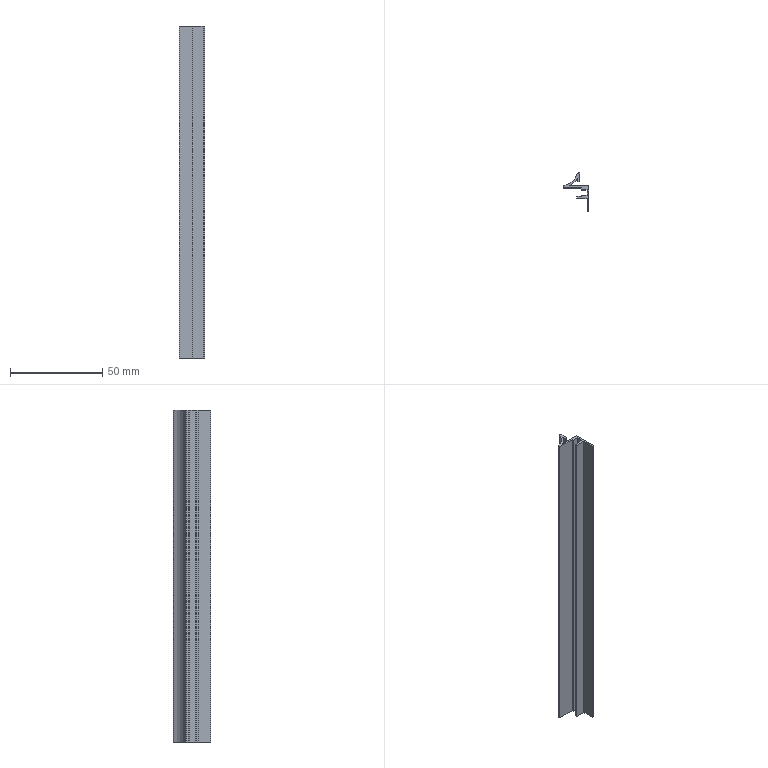Part | SolidWorks | features BaseBody 1, ICE 1, MoveFace 1 | 1 solid | 27 faces | box 14 x 20.3 x 180 mm | volume 9165 mm3 | plane 20 | cylinder 7 | commonest cylinder face diameters 0.387 x2 0.8 x2 0.4 x1 20 x1 22 x1
STEP:
#1=CARTESIAN_POINT('',(-5.304,-0.625,200.));
#2=VERTEX_POINT('',#1);
#3=CARTESIAN_POINT('',(-5.449,-0.8125,200.));
#4=VERTEX_POINT('',#3);
#5=CARTESIAN_POINT('',(-5.255,-0.8125,200.));
#6=DIRECTION('',(0.,0.,1.));
#7=DIRECTION('',(-1.,0.,0.));
#8=AXIS2_PLACEMENT_3D('',#5,#6,#7);
#9=CIRCLE('',#8,0.1937);
#10=EDGE_CURVE('',#2,#4,#9,.T.);
#11=ORIENTED_EDGE('',*,*,#10,.T.);
#12=CARTESIAN_POINT('',(-5.449,-0.8125,20.));
#13=VERTEX_POINT('',#12);
#14=CARTESIAN_POINT('',(-5.449,-0.8125,230.));
#15=DIRECTION('',(0.,0.,-1.));
#16=VECTOR('',#15,1000.);
#17=LINE('',#14,#16);
#18=EDGE_CURVE('',#4,#13,#17,.T.);
#19=ORIENTED_EDGE('',*,*,#18,.T.);
#20=CARTESIAN_POINT('',(-5.304,-0.625,20.));
#21=VERTEX_POINT('',#20);
#22=CARTESIAN_POINT('',(-5.255,-0.8125,20.));
#23=DIRECTION('',(0.,0.,-1.));
#24=DIRECTION('',(1.,0.,0.));
#25=AXIS2_PLACEMENT_3D('',#22,#23,#24);
#26=CIRCLE('',#25,0.1937);
#27=EDGE_CURVE('',#13,#21,#26,.T.);
#28=ORIENTED_EDGE('',*,*,#27,.T.);
#29=CARTESIAN_POINT('',(-5.304,-0.625,230.));
#30=DIRECTION('',(0.,0.,-1.));
#31=VECTOR('',#30,1000.);
#32=LINE('',#29,#31);
#33=EDGE_CURVE('',#2,#21,#32,.T.);
#34=ORIENTED_EDGE('',*,*,#33,.F.);
#35=EDGE_LOOP('',(#11,#19,#28,#34));
#36=FACE_OUTER_BOUND('',#35,.T.);
#37=CARTESIAN_POINT('',(-5.255,-0.8125,230.));
#38=DIRECTION('',(0.,0.,-1.));
#39=DIRECTION('',(-1.,0.,0.));
#40=AXIS2_PLACEMENT_3D('',#37,#38,#39);
#41=CYLINDRICAL_SURFACE('',#40,0.1937);
#42=ADVANCED_FACE('',(#36),#41,.F.);
#43=CARTESIAN_POINT('',(5.,-1.,20.));
#44=VERTEX_POINT('',#43);
#45=CARTESIAN_POINT('',(5.,-14.3,20.));
#46=VERTEX_POINT('',#45);
#47=CARTESIAN_POINT('',(5.,29.623,20.));
#48=DIRECTION('',(0.,-1.,0.));
#49=VECTOR('',#48,1000.);
#50=LINE('',#47,#49);
#51=EDGE_CURVE('',#44,#46,#50,.T.);
#52=ORIENTED_EDGE('',*,*,#51,.F.);
#53=CARTESIAN_POINT('',(5.,-1.,200.));
#54=VERTEX_POINT('',#53);
#55=CARTESIAN_POINT('',(5.,-1.,230.));
#56=DIRECTION('',(0.,0.,-1.));
#57=VECTOR('',#56,1000.);
#58=LINE('',#55,#57);
#59=EDGE_CURVE('',#54,#44,#58,.T.);
#60=ORIENTED_EDGE('',*,*,#59,.F.);
#61=CARTESIAN_POINT('',(5.,-14.3,200.));
#62=VERTEX_POINT('',#61);
#63=CARTESIAN_POINT('',(5.,-14.3,200.));
#64=DIRECTION('',(0.,1.,0.));
#65=VECTOR('',#64,1000.);
#66=LINE('',#63,#65);
#67=EDGE_CURVE('',#62,#54,#66,.T.);
#68=ORIENTED_EDGE('',*,*,#67,.F.);
#69=CARTESIAN_POINT('',(5.,-14.3,230.));
#70=DIRECTION('',(0.,0.,1.));
#71=VECTOR('',#70,1000.);
#72=LINE('',#69,#71);
#73=EDGE_CURVE('',#46,#62,#72,.T.);
#74=ORIENTED_EDGE('',*,*,#73,.F.);
#75=EDGE_LOOP('',(#52,#60,#68,#74));
#76=FACE_OUTER_BOUND('',#75,.T.);
#77=CARTESIAN_POINT('',(5.,-14.3,230.));
#78=DIRECTION('',(-1.,0.,0.));
#79=DIRECTION('',(0.,0.,1.));
#80=AXIS2_PLACEMENT_3D('',#77,#78,#79);
#81=PLANE('',#80);
#82=ADVANCED_FACE('',(#76),#81,.F.);
#83=CARTESIAN_POINT('',(-9.,-2.,20.));
#84=VERTEX_POINT('',#83);
#85=CARTESIAN_POINT('',(-9.,-2.,200.));
#86=VERTEX_POINT('',#85);
#87=CARTESIAN_POINT('',(-9.,-2.,230.));
#88=DIRECTION('',(0.,0.,1.));
#89=VECTOR('',#88,1000.);
#90=LINE('',#87,#89);
#91=EDGE_CURVE('',#84,#86,#90,.T.);
#92=ORIENTED_EDGE('',*,*,#91,.F.);
#93=CARTESIAN_POINT('',(0.9,-2.,20.));
#94=VERTEX_POINT('',#93);
#95=CARTESIAN_POINT('',(5.,-2.,20.));
#96=DIRECTION('',(-1.,0.,0.));
#97=VECTOR('',#96,1000.);
#98=LINE('',#95,#97);
#99=EDGE_CURVE('',#94,#84,#98,.T.);
#100=ORIENTED_EDGE('',*,*,#99,.F.);
#101=CARTESIAN_POINT('',(0.9,-2.,200.));
#102=VERTEX_POINT('',#101);
#103=CARTESIAN_POINT('',(0.9,-2.,230.));
#104=DIRECTION('',(0.,0.,-1.));
#105=VECTOR('',#104,1000.);
#106=LINE('',#103,#105);
#107=EDGE_CURVE('',#102,#94,#106,.T.);
#108=ORIENTED_EDGE('',*,*,#107,.F.);
#109=CARTESIAN_POINT('',(5.,-2.,200.));
#110=DIRECTION('',(1.,0.,0.));
#111=VECTOR('',#110,1000.);
#112=LINE('',#109,#111);
#113=EDGE_CURVE('',#86,#102,#112,.T.);
#114=ORIENTED_EDGE('',*,*,#113,.F.);
#115=EDGE_LOOP('',(#92,#100,#108,#114));
#116=FACE_OUTER_BOUND('',#115,.T.);
#117=CARTESIAN_POINT('',(-9.,-2.,230.));
#118=DIRECTION('',(0.,1.,0.));
#119=DIRECTION('',(0.,0.,1.));
#120=AXIS2_PLACEMENT_3D('',#117,#118,#119);
#121=PLANE('',#120);
#122=ADVANCED_FACE('',(#116),#121,.F.);
#123=CARTESIAN_POINT('',(4.,-6.,200.));
#124=VERTEX_POINT('',#123);
#125=CARTESIAN_POINT('',(4.,-3.,200.));
#126=VERTEX_POINT('',#125);
#127=CARTESIAN_POINT('',(4.,29.623,200.));
#128=DIRECTION('',(0.,1.,0.));
#129=VECTOR('',#128,1000.);
#130=LINE('',#127,#129);
#131=EDGE_CURVE('',#124,#126,#130,.T.);
#132=ORIENTED_EDGE('',*,*,#131,.F.);
#133=CARTESIAN_POINT('',(1.,-6.,200.));
#134=VERTEX_POINT('',#133);
#135=CARTESIAN_POINT('',(5.,-6.,200.));
#136=DIRECTION('',(1.,0.,0.));
#137=VECTOR('',#136,1000.);
#138=LINE('',#135,#137);
#139=EDGE_CURVE('',#134,#124,#138,.T.);
#140=ORIENTED_EDGE('',*,*,#139,.F.);
#141=CARTESIAN_POINT('',(1.,-6.7,200.));
#142=VERTEX_POINT('',#141);
#143=CARTESIAN_POINT('',(1.,-6.,200.));
#144=DIRECTION('',(0.,-1.,0.));
#145=VECTOR('',#144,1000.);
#146=LINE('',#143,#145);
#147=EDGE_CURVE('',#134,#142,#146,.T.);
#148=ORIENTED_EDGE('',*,*,#147,.T.);
#149=CARTESIAN_POINT('',(-1.7,-6.7,200.));
#150=VERTEX_POINT('',#149);
#151=CARTESIAN_POINT('',(5.,-6.7,200.));
#152=DIRECTION('',(1.,0.,0.));
#153=VECTOR('',#152,1000.);
#154=LINE('',#151,#153);
#155=EDGE_CURVE('',#150,#142,#154,.T.);
#156=ORIENTED_EDGE('',*,*,#155,.F.);
#157=CARTESIAN_POINT('',(-1.7,-7.7,200.));
#158=VERTEX_POINT('',#157);
#159=CARTESIAN_POINT('',(-1.7,-6.7,200.));
#160=DIRECTION('',(0.,-1.,0.));
#161=VECTOR('',#160,1000.);
#162=LINE('',#159,#161);
#163=EDGE_CURVE('',#150,#158,#162,.T.);
#164=ORIENTED_EDGE('',*,*,#163,.T.);
#165=CARTESIAN_POINT('',(4.,-7.7,200.));
#166=VERTEX_POINT('',#165);
#167=CARTESIAN_POINT('',(5.,-7.7,200.));
#168=DIRECTION('',(-1.,0.,0.));
#169=VECTOR('',#168,1000.);
#170=LINE('',#167,#169);
#171=EDGE_CURVE('',#166,#158,#170,.T.);
#172=ORIENTED_EDGE('',*,*,#171,.F.);
#173=CARTESIAN_POINT('',(4.,-14.3,200.));
#174=VERTEX_POINT('',#173);
#175=CARTESIAN_POINT('',(4.,29.623,200.));
#176=DIRECTION('',(0.,1.,0.));
#177=VECTOR('',#176,1000.);
#178=LINE('',#175,#177);
#179=EDGE_CURVE('',#174,#166,#178,.T.);
#180=ORIENTED_EDGE('',*,*,#179,.F.);
#181=CARTESIAN_POINT('',(5.,-14.3,200.));
#182=DIRECTION('',(-1.,0.,0.));
#183=VECTOR('',#182,1000.);
#184=LINE('',#181,#183);
#185=EDGE_CURVE('',#62,#174,#184,.T.);
#186=ORIENTED_EDGE('',*,*,#185,.F.);
#187=ORIENTED_EDGE('',*,*,#67,.T.);
#188=CARTESIAN_POINT('',(-5.207,-1.,200.));
#189=VERTEX_POINT('',#188);
#190=CARTESIAN_POINT('',(5.,-1.,200.));
#191=DIRECTION('',(1.,0.,0.));
#192=VECTOR('',#191,1000.);
#193=LINE('',#190,#192);
#194=EDGE_CURVE('',#189,#54,#193,.T.);
#195=ORIENTED_EDGE('',*,*,#194,.F.);
#196=CARTESIAN_POINT('',(-5.255,-0.8125,200.));
#197=DIRECTION('',(0.,0.,1.));
#198=DIRECTION('',(-1.,0.,0.));
#199=AXIS2_PLACEMENT_3D('',#196,#197,#198);
#200=CIRCLE('',#199,0.1937);
#201=EDGE_CURVE('',#4,#189,#200,.T.);
#202=ORIENTED_EDGE('',*,*,#201,.F.);
#203=ORIENTED_EDGE('',*,*,#10,.F.);
#204=CARTESIAN_POINT('',(-1.368,3.063,200.));
#205=VERTEX_POINT('',#204);
#206=CARTESIAN_POINT('',(-10.628,9.,200.));
#207=DIRECTION('',(0.,0.,1.));
#208=DIRECTION('',(-1.,0.,0.));
#209=AXIS2_PLACEMENT_3D('',#206,#207,#208);
#210=CIRCLE('',#209,11.);
#211=EDGE_CURVE('',#2,#205,#210,.T.);
#212=ORIENTED_EDGE('',*,*,#211,.T.);
#213=CARTESIAN_POINT('',(-1.,2.955,200.));
#214=VERTEX_POINT('',#213);
#215=CARTESIAN_POINT('',(-1.2,2.955,200.));
#216=DIRECTION('',(0.,0.,1.));
#217=DIRECTION('',(-1.,0.,0.));
#218=AXIS2_PLACEMENT_3D('',#215,#216,#217);
#219=CIRCLE('',#218,0.2);
#220=EDGE_CURVE('',#214,#205,#219,.T.);
#221=ORIENTED_EDGE('',*,*,#220,.F.);
#222=CARTESIAN_POINT('',(-1.,1.5,200.));
#223=VERTEX_POINT('',#222);
#224=CARTESIAN_POINT('',(-1.,2.955,200.));
#225=DIRECTION('',(0.,1.,0.));
#226=VECTOR('',#225,1000.);
#227=LINE('',#224,#226);
#228=EDGE_CURVE('',#223,#214,#227,.T.);
#229=ORIENTED_EDGE('',*,*,#228,.F.);
#230=CARTESIAN_POINT('',(0.,1.5,200.));
#231=VERTEX_POINT('',#230);
#232=CARTESIAN_POINT('',(-1.,1.5,200.));
#233=DIRECTION('',(-1.,0.,0.));
#234=VECTOR('',#233,1000.);
#235=LINE('',#232,#234);
#236=EDGE_CURVE('',#231,#223,#235,.T.);
#237=ORIENTED_EDGE('',*,*,#236,.F.);
#238=CARTESIAN_POINT('',(0.,6.,200.));
#239=VERTEX_POINT('',#238);
#240=CARTESIAN_POINT('',(0.,1.5,200.));
#241=DIRECTION('',(0.,-1.,0.));
#242=VECTOR('',#241,1000.);
#243=LINE('',#240,#242);
#244=EDGE_CURVE('',#239,#231,#243,.T.);
#245=ORIENTED_EDGE('',*,*,#244,.F.);
#246=CARTESIAN_POINT('',(-0.8,6.,200.));
#247=VERTEX_POINT('',#246);
#248=CARTESIAN_POINT('',(0.,6.,200.));
#249=DIRECTION('',(1.,0.,0.));
#250=VECTOR('',#249,1000.);
#251=LINE('',#248,#250);
#252=EDGE_CURVE('',#247,#239,#251,.T.);
#253=ORIENTED_EDGE('',*,*,#252,.F.);
#254=CARTESIAN_POINT('',(-1.178,5.731,200.));
#255=VERTEX_POINT('',#254);
#256=CARTESIAN_POINT('',(-0.8,5.6,200.));
#257=DIRECTION('',(0.,0.,1.));
#258=DIRECTION('',(-1.,0.,0.));
#259=AXIS2_PLACEMENT_3D('',#256,#257,#258);
#260=CIRCLE('',#259,0.4);
#261=EDGE_CURVE('',#247,#255,#260,.T.);
#262=ORIENTED_EDGE('',*,*,#261,.T.);
#263=CARTESIAN_POINT('',(-8.678,-0.8077,200.));
#264=VERTEX_POINT('',#263);
#265=CARTESIAN_POINT('',(-10.628,9.,200.));
#266=DIRECTION('',(0.,0.,1.));
#267=DIRECTION('',(-1.,0.,0.));
#268=AXIS2_PLACEMENT_3D('',#265,#266,#267);
#269=CIRCLE('',#268,10.);
#270=EDGE_CURVE('',#264,#255,#269,.T.);
#271=ORIENTED_EDGE('',*,*,#270,.F.);
#272=CARTESIAN_POINT('',(-9.,-1.2,200.));
#273=VERTEX_POINT('',#272);
#274=CARTESIAN_POINT('',(-8.6,-1.2,200.));
#275=DIRECTION('',(0.,0.,1.));
#276=DIRECTION('',(-1.,0.,0.));
#277=AXIS2_PLACEMENT_3D('',#274,#275,#276);
#278=CIRCLE('',#277,0.4);
#279=EDGE_CURVE('',#264,#273,#278,.T.);
#280=ORIENTED_EDGE('',*,*,#279,.T.);
#281=CARTESIAN_POINT('',(-9.,8.,200.));
#282=DIRECTION('',(0.,-1.,0.));
#283=VECTOR('',#282,1000.);
#284=LINE('',#281,#283);
#285=EDGE_CURVE('',#273,#86,#284,.T.);
#286=ORIENTED_EDGE('',*,*,#285,.T.);
#287=ORIENTED_EDGE('',*,*,#113,.T.);
#288=CARTESIAN_POINT('',(0.9,-3.,200.));
#289=VERTEX_POINT('',#288);
#290=CARTESIAN_POINT('',(0.9,29.623,200.));
#291=DIRECTION('',(0.,1.,0.));
#292=VECTOR('',#291,1000.);
#293=LINE('',#290,#292);
#294=EDGE_CURVE('',#289,#102,#293,.T.);
#295=ORIENTED_EDGE('',*,*,#294,.F.);
#296=CARTESIAN_POINT('',(5.,-3.,200.));
#297=DIRECTION('',(-1.,0.,0.));
#298=VECTOR('',#297,1000.);
#299=LINE('',#296,#298);
#300=EDGE_CURVE('',#126,#289,#299,.T.);
#301=ORIENTED_EDGE('',*,*,#300,.F.);
#302=EDGE_LOOP('',(#132,#140,#148,#156,#164,#172,#180,#186,#187,#195,#202,#203,#212,#221,#229,#237,#245,#253,#262,#271,#280,#286,#287,#295,#301));
#303=FACE_OUTER_BOUND('',#302,.T.);
#304=CARTESIAN_POINT('',(5.,29.623,200.));
#305=DIRECTION('',(0.,0.,-1.));
#306=DIRECTION('',(-1.,0.,0.));
#307=AXIS2_PLACEMENT_3D('',#304,#305,#306);
#308=PLANE('',#307);
#309=ADVANCED_FACE('',(#303),#308,.F.);
#310=ORIENTED_EDGE('',*,*,#185,.T.);
#311=CARTESIAN_POINT('',(4.,-14.3,20.));
#312=VERTEX_POINT('',#311);
#313=CARTESIAN_POINT('',(4.,-14.3,230.));
#314=DIRECTION('',(0.,0.,1.));
#315=VECTOR('',#314,1000.);
#316=LINE('',#313,#315);
#317=EDGE_CURVE('',#312,#174,#316,.T.);
#318=ORIENTED_EDGE('',*,*,#317,.F.);
#319=CARTESIAN_POINT('',(5.,-14.3,20.));
#320=DIRECTION('',(-1.,0.,0.));
#321=VECTOR('',#320,1000.);
#322=LINE('',#319,#321);
#323=EDGE_CURVE('',#46,#312,#322,.T.);
#324=ORIENTED_EDGE('',*,*,#323,.F.);
#325=ORIENTED_EDGE('',*,*,#73,.T.);
#326=EDGE_LOOP('',(#310,#318,#324,#325));
#327=FACE_OUTER_BOUND('',#326,.T.);
#328=CARTESIAN_POINT('',(4.,-14.3,230.));
#329=DIRECTION('',(0.,1.,0.));
#330=DIRECTION('',(0.,0.,1.));
#331=AXIS2_PLACEMENT_3D('',#328,#329,#330);
#332=PLANE('',#331);
#333=ADVANCED_FACE('',(#327),#332,.F.);
#334=ORIENTED_EDGE('',*,*,#51,.T.);
#335=ORIENTED_EDGE('',*,*,#323,.T.);
#336=CARTESIAN_POINT('',(4.,-7.7,20.));
#337=VERTEX_POINT('',#336);
#338=CARTESIAN_POINT('',(4.,-7.7,20.));
#339=DIRECTION('',(0.,-1.,0.));
#340=VECTOR('',#339,1000.);
#341=LINE('',#338,#340);
#342=EDGE_CURVE('',#337,#312,#341,.T.);
#343=ORIENTED_EDGE('',*,*,#342,.F.);
#344=CARTESIAN_POINT('',(-1.7,-7.7,20.));
#345=VERTEX_POINT('',#344);
#346=CARTESIAN_POINT('',(-1.7,-7.7,20.));
#347=DIRECTION('',(1.,0.,0.));
#348=VECTOR('',#347,1000.);
#349=LINE('',#346,#348);
#350=EDGE_CURVE('',#345,#337,#349,.T.);
#351=ORIENTED_EDGE('',*,*,#350,.F.);
#352=CARTESIAN_POINT('',(-1.7,-6.7,20.));
#353=VERTEX_POINT('',#352);
#354=CARTESIAN_POINT('',(-1.7,29.623,20.));
#355=DIRECTION('',(0.,1.,0.));
#356=VECTOR('',#355,1000.);
#357=LINE('',#354,#356);
#358=EDGE_CURVE('',#345,#353,#357,.T.);
#359=ORIENTED_EDGE('',*,*,#358,.T.);
#360=CARTESIAN_POINT('',(1.,-6.7,20.));
#361=VERTEX_POINT('',#360);
#362=CARTESIAN_POINT('',(1.,-6.7,20.));
#363=DIRECTION('',(-1.,0.,0.));
#364=VECTOR('',#363,1000.);
#365=LINE('',#362,#364);
#366=EDGE_CURVE('',#361,#353,#365,.T.);
#367=ORIENTED_EDGE('',*,*,#366,.F.);
#368=CARTESIAN_POINT('',(1.,-6.,20.));
#369=VERTEX_POINT('',#368);
#370=CARTESIAN_POINT('',(1.,29.623,20.));
#371=DIRECTION('',(0.,1.,0.));
#372=VECTOR('',#371,1000.);
#373=LINE('',#370,#372);
#374=EDGE_CURVE('',#361,#369,#373,.T.);
#375=ORIENTED_EDGE('',*,*,#374,.T.);
#376=CARTESIAN_POINT('',(4.,-6.,20.));
#377=VERTEX_POINT('',#376);
#378=CARTESIAN_POINT('',(4.,-6.,20.));
#379=DIRECTION('',(-1.,0.,0.));
#380=VECTOR('',#379,1000.);
#381=LINE('',#378,#380);
#382=EDGE_CURVE('',#377,#369,#381,.T.);
#383=ORIENTED_EDGE('',*,*,#382,.F.);
#384=CARTESIAN_POINT('',(4.,-3.,20.));
#385=VERTEX_POINT('',#384);
#386=CARTESIAN_POINT('',(4.,-3.,20.));
#387=DIRECTION('',(0.,-1.,0.));
#388=VECTOR('',#387,1000.);
#389=LINE('',#386,#388);
#390=EDGE_CURVE('',#385,#377,#389,.T.);
#391=ORIENTED_EDGE('',*,*,#390,.F.);
#392=CARTESIAN_POINT('',(0.9,-3.,20.));
#393=VERTEX_POINT('',#392);
#394=CARTESIAN_POINT('',(0.9,-3.,20.));
#395=DIRECTION('',(1.,0.,0.));
#396=VECTOR('',#395,1000.);
#397=LINE('',#394,#396);
#398=EDGE_CURVE('',#393,#385,#397,.T.);
#399=ORIENTED_EDGE('',*,*,#398,.F.);
#400=CARTESIAN_POINT('',(0.9,-2.,20.));
#401=DIRECTION('',(0.,-1.,0.));
#402=VECTOR('',#401,1000.);
#403=LINE('',#400,#402);
#404=EDGE_CURVE('',#94,#393,#403,.T.);
#405=ORIENTED_EDGE('',*,*,#404,.F.);
#406=ORIENTED_EDGE('',*,*,#99,.T.);
#407=CARTESIAN_POINT('',(-9.,-1.2,20.));
#408=VERTEX_POINT('',#407);
#409=CARTESIAN_POINT('',(-9.,-1.2,20.));
#410=DIRECTION('',(0.,-1.,0.));
#411=VECTOR('',#410,1000.);
#412=LINE('',#409,#411);
#413=EDGE_CURVE('',#408,#84,#412,.T.);
#414=ORIENTED_EDGE('',*,*,#413,.F.);
#415=CARTESIAN_POINT('',(-8.678,-0.8077,20.));
#416=VERTEX_POINT('',#415);
#417=CARTESIAN_POINT('',(-8.6,-1.2,20.));
#418=DIRECTION('',(0.,0.,-1.));
#419=DIRECTION('',(1.,0.,0.));
#420=AXIS2_PLACEMENT_3D('',#417,#418,#419);
#421=CIRCLE('',#420,0.4);
#422=EDGE_CURVE('',#408,#416,#421,.T.);
#423=ORIENTED_EDGE('',*,*,#422,.T.);
#424=CARTESIAN_POINT('',(-1.178,5.731,20.));
#425=VERTEX_POINT('',#424);
#426=CARTESIAN_POINT('',(-10.628,9.,20.));
#427=DIRECTION('',(0.,0.,-1.));
#428=DIRECTION('',(1.,0.,0.));
#429=AXIS2_PLACEMENT_3D('',#426,#427,#428);
#430=CIRCLE('',#429,10.);
#431=EDGE_CURVE('',#425,#416,#430,.T.);
#432=ORIENTED_EDGE('',*,*,#431,.F.);
#433=CARTESIAN_POINT('',(-0.8,6.,20.));
#434=VERTEX_POINT('',#433);
#435=CARTESIAN_POINT('',(-0.8,5.6,20.));
#436=DIRECTION('',(0.,0.,-1.));
#437=DIRECTION('',(1.,0.,0.));
#438=AXIS2_PLACEMENT_3D('',#435,#436,#437);
#439=CIRCLE('',#438,0.4);
#440=EDGE_CURVE('',#425,#434,#439,.T.);
#441=ORIENTED_EDGE('',*,*,#440,.T.);
#442=CARTESIAN_POINT('',(0.,6.,20.));
#443=VERTEX_POINT('',#442);
#444=CARTESIAN_POINT('',(0.,6.,20.));
#445=DIRECTION('',(-1.,0.,0.));
#446=VECTOR('',#445,1000.);
#447=LINE('',#444,#446);
#448=EDGE_CURVE('',#443,#434,#447,.T.);
#449=ORIENTED_EDGE('',*,*,#448,.F.);
#450=CARTESIAN_POINT('',(0.,1.5,20.));
#451=VERTEX_POINT('',#450);
#452=CARTESIAN_POINT('',(0.,1.5,20.));
#453=DIRECTION('',(0.,1.,0.));
#454=VECTOR('',#453,1000.);
#455=LINE('',#452,#454);
#456=EDGE_CURVE('',#451,#443,#455,.T.);
#457=ORIENTED_EDGE('',*,*,#456,.F.);
#458=CARTESIAN_POINT('',(-1.,1.5,20.));
#459=VERTEX_POINT('',#458);
#460=CARTESIAN_POINT('',(-1.,1.5,20.));
#461=DIRECTION('',(1.,0.,0.));
#462=VECTOR('',#461,1000.);
#463=LINE('',#460,#462);
#464=EDGE_CURVE('',#459,#451,#463,.T.);
#465=ORIENTED_EDGE('',*,*,#464,.F.);
#466=CARTESIAN_POINT('',(-1.,2.955,20.));
#467=VERTEX_POINT('',#466);
#468=CARTESIAN_POINT('',(-1.,2.955,20.));
#469=DIRECTION('',(0.,-1.,0.));
#470=VECTOR('',#469,1000.);
#471=LINE('',#468,#470);
#472=EDGE_CURVE('',#467,#459,#471,.T.);
#473=ORIENTED_EDGE('',*,*,#472,.F.);
#474=CARTESIAN_POINT('',(-1.368,3.063,20.));
#475=VERTEX_POINT('',#474);
#476=CARTESIAN_POINT('',(-1.2,2.955,20.));
#477=DIRECTION('',(0.,0.,-1.));
#478=DIRECTION('',(1.,0.,0.));
#479=AXIS2_PLACEMENT_3D('',#476,#477,#478);
#480=CIRCLE('',#479,0.2);
#481=EDGE_CURVE('',#475,#467,#480,.T.);
#482=ORIENTED_EDGE('',*,*,#481,.F.);
#483=CARTESIAN_POINT('',(-10.628,9.,20.));
#484=DIRECTION('',(0.,0.,-1.));
#485=DIRECTION('',(1.,0.,0.));
#486=AXIS2_PLACEMENT_3D('',#483,#484,#485);
#487=CIRCLE('',#486,11.);
#488=EDGE_CURVE('',#475,#21,#487,.T.);
#489=ORIENTED_EDGE('',*,*,#488,.T.);
#490=ORIENTED_EDGE('',*,*,#27,.F.);
#491=CARTESIAN_POINT('',(-5.207,-1.,20.));
#492=VERTEX_POINT('',#491);
#493=CARTESIAN_POINT('',(-5.255,-0.8125,20.));
#494=DIRECTION('',(0.,0.,-1.));
#495=DIRECTION('',(1.,0.,0.));
#496=AXIS2_PLACEMENT_3D('',#493,#494,#495);
#497=CIRCLE('',#496,0.1937);
#498=EDGE_CURVE('',#492,#13,#497,.T.);
#499=ORIENTED_EDGE('',*,*,#498,.F.);
#500=CARTESIAN_POINT('',(5.,-1.,20.));
#501=DIRECTION('',(-1.,0.,0.));
#502=VECTOR('',#501,1000.);
#503=LINE('',#500,#502);
#504=EDGE_CURVE('',#44,#492,#503,.T.);
#505=ORIENTED_EDGE('',*,*,#504,.F.);
#506=EDGE_LOOP('',(#334,#335,#343,#351,#359,#367,#375,#383,#391,#399,#405,#406,#414,#423,#432,#441,#449,#457,#465,#473,#482,#489,#490,#499,#505));
#507=FACE_OUTER_BOUND('',#506,.T.);
#508=CARTESIAN_POINT('',(5.,29.623,20.));
#509=DIRECTION('',(0.,0.,1.));
#510=DIRECTION('',(1.,0.,0.));
#511=AXIS2_PLACEMENT_3D('',#508,#509,#510);
#512=PLANE('',#511);
#513=ADVANCED_FACE('',(#507),#512,.F.);
#514=ORIENTED_EDGE('',*,*,#59,.T.);
#515=ORIENTED_EDGE('',*,*,#504,.T.);
#516=CARTESIAN_POINT('',(-5.207,-1.,230.));
#517=DIRECTION('',(0.,0.,-1.));
#518=VECTOR('',#517,1000.);
#519=LINE('',#516,#518);
#520=EDGE_CURVE('',#189,#492,#519,.T.);
#521=ORIENTED_EDGE('',*,*,#520,.F.);
#522=ORIENTED_EDGE('',*,*,#194,.T.);
#523=EDGE_LOOP('',(#514,#515,#521,#522));
#524=FACE_OUTER_BOUND('',#523,.T.);
#525=CARTESIAN_POINT('',(5.,-1.,230.));
#526=DIRECTION('',(0.,-1.,0.));
#527=DIRECTION('',(0.,0.,-1.));
#528=AXIS2_PLACEMENT_3D('',#525,#526,#527);
#529=PLANE('',#528);
#530=ADVANCED_FACE('',(#524),#529,.F.);
#531=CARTESIAN_POINT('',(-9.,-1.2,230.));
#532=DIRECTION('',(0.,0.,1.));
#533=VECTOR('',#532,1000.);
#534=LINE('',#531,#533);
#535=EDGE_CURVE('',#408,#273,#534,.T.);
#536=ORIENTED_EDGE('',*,*,#535,.F.);
#537=ORIENTED_EDGE('',*,*,#413,.T.);
#538=ORIENTED_EDGE('',*,*,#91,.T.);
#539=ORIENTED_EDGE('',*,*,#285,.F.);
#540=EDGE_LOOP('',(#536,#537,#538,#539));
#541=FACE_OUTER_BOUND('',#540,.T.);
#542=CARTESIAN_POINT('',(-9.,-1.2,230.));
#543=DIRECTION('',(1.,0.,0.));
#544=DIRECTION('',(0.,0.,-1.));
#545=AXIS2_PLACEMENT_3D('',#542,#543,#544);
#546=PLANE('',#545);
#547=ADVANCED_FACE('',(#541),#546,.F.);
#548=ORIENTED_EDGE('',*,*,#294,.T.);
#549=ORIENTED_EDGE('',*,*,#107,.T.);
#550=ORIENTED_EDGE('',*,*,#404,.T.);
#551=CARTESIAN_POINT('',(0.9,-3.,230.));
#552=DIRECTION('',(0.,0.,-1.));
#553=VECTOR('',#552,1000.);
#554=LINE('',#551,#553);
#555=EDGE_CURVE('',#289,#393,#554,.T.);
#556=ORIENTED_EDGE('',*,*,#555,.F.);
#557=EDGE_LOOP('',(#548,#549,#550,#556));
#558=FACE_OUTER_BOUND('',#557,.T.);
#559=CARTESIAN_POINT('',(0.9,-2.,230.));
#560=DIRECTION('',(1.,0.,0.));
#561=DIRECTION('',(0.,0.,-1.));
#562=AXIS2_PLACEMENT_3D('',#559,#560,#561);
#563=PLANE('',#562);
#564=ADVANCED_FACE('',(#558),#563,.F.);
#565=ORIENTED_EDGE('',*,*,#300,.T.);
#566=ORIENTED_EDGE('',*,*,#555,.T.);
#567=ORIENTED_EDGE('',*,*,#398,.T.);
#568=CARTESIAN_POINT('',(4.,-3.,230.));
#569=DIRECTION('',(0.,0.,-1.));
#570=VECTOR('',#569,1000.);
#571=LINE('',#568,#570);
#572=EDGE_CURVE('',#126,#385,#571,.T.);
#573=ORIENTED_EDGE('',*,*,#572,.F.);
#574=EDGE_LOOP('',(#565,#566,#567,#573));
#575=FACE_OUTER_BOUND('',#574,.T.);
#576=CARTESIAN_POINT('',(0.9,-3.,230.));
#577=DIRECTION('',(0.,1.,0.));
#578=DIRECTION('',(0.,0.,1.));
#579=AXIS2_PLACEMENT_3D('',#576,#577,#578);
#580=PLANE('',#579);
#581=ADVANCED_FACE('',(#575),#580,.F.);
#582=ORIENTED_EDGE('',*,*,#131,.T.);
#583=ORIENTED_EDGE('',*,*,#572,.T.);
#584=ORIENTED_EDGE('',*,*,#390,.T.);
#585=CARTESIAN_POINT('',(4.,-6.,230.));
#586=DIRECTION('',(0.,0.,-1.));
#587=VECTOR('',#586,1000.);
#588=LINE('',#585,#587);
#589=EDGE_CURVE('',#124,#377,#588,.T.);
#590=ORIENTED_EDGE('',*,*,#589,.F.);
#591=EDGE_LOOP('',(#582,#583,#584,#590));
#592=FACE_OUTER_BOUND('',#591,.T.);
#593=CARTESIAN_POINT('',(4.,-3.,230.));
#594=DIRECTION('',(1.,0.,0.));
#595=DIRECTION('',(0.,0.,-1.));
#596=AXIS2_PLACEMENT_3D('',#593,#594,#595);
#597=PLANE('',#596);
#598=ADVANCED_FACE('',(#592),#597,.F.);
#599=ORIENTED_EDGE('',*,*,#139,.T.);
#600=ORIENTED_EDGE('',*,*,#589,.T.);
#601=ORIENTED_EDGE('',*,*,#382,.T.);
#602=CARTESIAN_POINT('',(1.,-6.,230.));
#603=DIRECTION('',(0.,0.,-1.));
#604=VECTOR('',#603,1000.);
#605=LINE('',#602,#604);
#606=EDGE_CURVE('',#134,#369,#605,.T.);
#607=ORIENTED_EDGE('',*,*,#606,.F.);
#608=EDGE_LOOP('',(#599,#600,#601,#607));
#609=FACE_OUTER_BOUND('',#608,.T.);
#610=CARTESIAN_POINT('',(4.,-6.,230.));
#611=DIRECTION('',(0.,-1.,0.));
#612=DIRECTION('',(0.,0.,-1.));
#613=AXIS2_PLACEMENT_3D('',#610,#611,#612);
#614=PLANE('',#613);
#615=ADVANCED_FACE('',(#609),#614,.F.);
#616=ORIENTED_EDGE('',*,*,#155,.T.);
#617=CARTESIAN_POINT('',(1.,-6.7,230.));
#618=DIRECTION('',(0.,0.,1.));
#619=VECTOR('',#618,1000.);
#620=LINE('',#617,#619);
#621=EDGE_CURVE('',#361,#142,#620,.T.);
#622=ORIENTED_EDGE('',*,*,#621,.F.);
#623=ORIENTED_EDGE('',*,*,#366,.T.);
#624=CARTESIAN_POINT('',(-1.7,-6.7,230.));
#625=DIRECTION('',(0.,0.,-1.));
#626=VECTOR('',#625,1000.);
#627=LINE('',#624,#626);
#628=EDGE_CURVE('',#150,#353,#627,.T.);
#629=ORIENTED_EDGE('',*,*,#628,.F.);
#630=EDGE_LOOP('',(#616,#622,#623,#629));
#631=FACE_OUTER_BOUND('',#630,.T.);
#632=CARTESIAN_POINT('',(1.,-6.7,230.));
#633=DIRECTION('',(0.,-1.,0.));
#634=DIRECTION('',(0.,0.,-1.));
#635=AXIS2_PLACEMENT_3D('',#632,#633,#634);
#636=PLANE('',#635);
#637=ADVANCED_FACE('',(#631),#636,.F.);
#638=ORIENTED_EDGE('',*,*,#171,.T.);
#639=CARTESIAN_POINT('',(-1.7,-7.7,230.));
#640=DIRECTION('',(0.,0.,1.));
#641=VECTOR('',#640,1000.);
#642=LINE('',#639,#641);
#643=EDGE_CURVE('',#345,#158,#642,.T.);
#644=ORIENTED_EDGE('',*,*,#643,.F.);
#645=ORIENTED_EDGE('',*,*,#350,.T.);
#646=CARTESIAN_POINT('',(4.,-7.7,230.));
#647=DIRECTION('',(0.,0.,-1.));
#648=VECTOR('',#647,1000.);
#649=LINE('',#646,#648);
#650=EDGE_CURVE('',#166,#337,#649,.T.);
#651=ORIENTED_EDGE('',*,*,#650,.F.);
#652=EDGE_LOOP('',(#638,#644,#645,#651));
#653=FACE_OUTER_BOUND('',#652,.T.);
#654=CARTESIAN_POINT('',(-1.7,-7.7,230.));
#655=DIRECTION('',(0.,1.,0.));
#656=DIRECTION('',(0.,0.,1.));
#657=AXIS2_PLACEMENT_3D('',#654,#655,#656);
#658=PLANE('',#657);
#659=ADVANCED_FACE('',(#653),#658,.F.);
#660=ORIENTED_EDGE('',*,*,#179,.T.);
#661=ORIENTED_EDGE('',*,*,#650,.T.);
#662=ORIENTED_EDGE('',*,*,#342,.T.);
#663=ORIENTED_EDGE('',*,*,#317,.T.);
#664=EDGE_LOOP('',(#660,#661,#662,#663));
#665=FACE_OUTER_BOUND('',#664,.T.);
#666=CARTESIAN_POINT('',(4.,-7.7,230.));
#667=DIRECTION('',(1.,0.,0.));
#668=DIRECTION('',(0.,0.,-1.));
#669=AXIS2_PLACEMENT_3D('',#666,#667,#668);
#670=PLANE('',#669);
#671=ADVANCED_FACE('',(#665),#670,.F.);
#672=ORIENTED_EDGE('',*,*,#18,.F.);
#673=ORIENTED_EDGE('',*,*,#201,.T.);
#674=ORIENTED_EDGE('',*,*,#520,.T.);
#675=ORIENTED_EDGE('',*,*,#498,.T.);
#676=EDGE_LOOP('',(#672,#673,#674,#675));
#677=FACE_OUTER_BOUND('',#676,.T.);
#678=CARTESIAN_POINT('',(-5.255,-0.8125,230.));
#679=DIRECTION('',(0.,0.,-1.));
#680=DIRECTION('',(-1.,0.,0.));
#681=AXIS2_PLACEMENT_3D('',#678,#679,#680);
#682=CYLINDRICAL_SURFACE('',#681,0.1937);
#683=ADVANCED_FACE('',(#677),#682,.F.);
#684=CARTESIAN_POINT('',(-1.,2.955,230.));
#685=DIRECTION('',(0.,0.,1.));
#686=VECTOR('',#685,1000.);
#687=LINE('',#684,#686);
#688=EDGE_CURVE('',#467,#214,#687,.T.);
#689=ORIENTED_EDGE('',*,*,#688,.F.);
#690=ORIENTED_EDGE('',*,*,#472,.T.);
#691=CARTESIAN_POINT('',(-1.,1.5,230.));
#692=DIRECTION('',(0.,0.,-1.));
#693=VECTOR('',#692,1000.);
#694=LINE('',#691,#693);
#695=EDGE_CURVE('',#223,#459,#694,.T.);
#696=ORIENTED_EDGE('',*,*,#695,.F.);
#697=ORIENTED_EDGE('',*,*,#228,.T.);
#698=EDGE_LOOP('',(#689,#690,#696,#697));
#699=FACE_OUTER_BOUND('',#698,.T.);
#700=CARTESIAN_POINT('',(-1.,2.955,230.));
#701=DIRECTION('',(1.,0.,0.));
#702=DIRECTION('',(0.,0.,-1.));
#703=AXIS2_PLACEMENT_3D('',#700,#701,#702);
#704=PLANE('',#703);
#705=ADVANCED_FACE('',(#699),#704,.F.);
#706=ORIENTED_EDGE('',*,*,#488,.F.);
#707=CARTESIAN_POINT('',(-1.368,3.063,230.));
#708=DIRECTION('',(0.,0.,1.));
#709=VECTOR('',#708,1000.);
#710=LINE('',#707,#709);
#711=EDGE_CURVE('',#475,#205,#710,.T.);
#712=ORIENTED_EDGE('',*,*,#711,.T.);
#713=ORIENTED_EDGE('',*,*,#211,.F.);
#714=ORIENTED_EDGE('',*,*,#33,.T.);
#715=EDGE_LOOP('',(#706,#712,#713,#714));
#716=FACE_OUTER_BOUND('',#715,.T.);
#717=CARTESIAN_POINT('',(-10.628,9.,230.));
#718=DIRECTION('',(0.,0.,-1.));
#719=DIRECTION('',(-1.,0.,0.));
#720=AXIS2_PLACEMENT_3D('',#717,#718,#719);
#721=CYLINDRICAL_SURFACE('',#720,11.);
#722=ADVANCED_FACE('',(#716),#721,.T.);
#723=CARTESIAN_POINT('',(-1.178,5.731,230.));
#724=DIRECTION('',(0.,0.,1.));
#725=VECTOR('',#724,1000.);
#726=LINE('',#723,#725);
#727=EDGE_CURVE('',#425,#255,#726,.T.);
#728=ORIENTED_EDGE('',*,*,#727,.F.);
#729=ORIENTED_EDGE('',*,*,#431,.T.);
#730=CARTESIAN_POINT('',(-8.678,-0.8077,230.));
#731=DIRECTION('',(0.,0.,-1.));
#732=VECTOR('',#731,1000.);
#733=LINE('',#730,#732);
#734=EDGE_CURVE('',#264,#416,#733,.T.);
#735=ORIENTED_EDGE('',*,*,#734,.F.);
#736=ORIENTED_EDGE('',*,*,#270,.T.);
#737=EDGE_LOOP('',(#728,#729,#735,#736));
#738=FACE_OUTER_BOUND('',#737,.T.);
#739=CARTESIAN_POINT('',(-10.628,9.,230.));
#740=DIRECTION('',(0.,0.,-1.));
#741=DIRECTION('',(-1.,0.,0.));
#742=AXIS2_PLACEMENT_3D('',#739,#740,#741);
#743=CYLINDRICAL_SURFACE('',#742,10.);
#744=ADVANCED_FACE('',(#738),#743,.F.);
#745=CARTESIAN_POINT('',(0.,1.5,230.));
#746=DIRECTION('',(0.,0.,1.));
#747=VECTOR('',#746,1000.);
#748=LINE('',#745,#747);
#749=EDGE_CURVE('',#451,#231,#748,.T.);
#750=ORIENTED_EDGE('',*,*,#749,.F.);
#751=ORIENTED_EDGE('',*,*,#456,.T.);
#752=CARTESIAN_POINT('',(0.,6.,230.));
#753=DIRECTION('',(0.,0.,-1.));
#754=VECTOR('',#753,1000.);
#755=LINE('',#752,#754);
#756=EDGE_CURVE('',#239,#443,#755,.T.);
#757=ORIENTED_EDGE('',*,*,#756,.F.);
#758=ORIENTED_EDGE('',*,*,#244,.T.);
#759=EDGE_LOOP('',(#750,#751,#757,#758));
#760=FACE_OUTER_BOUND('',#759,.T.);
#761=CARTESIAN_POINT('',(0.,1.5,230.));
#762=DIRECTION('',(-1.,0.,0.));
#763=DIRECTION('',(0.,0.,1.));
#764=AXIS2_PLACEMENT_3D('',#761,#762,#763);
#765=PLANE('',#764);
#766=ADVANCED_FACE('',(#760),#765,.F.);
#767=ORIENTED_EDGE('',*,*,#422,.F.);
#768=ORIENTED_EDGE('',*,*,#535,.T.);
#769=ORIENTED_EDGE('',*,*,#279,.F.);
#770=ORIENTED_EDGE('',*,*,#734,.T.);
#771=EDGE_LOOP('',(#767,#768,#769,#770));
#772=FACE_OUTER_BOUND('',#771,.T.);
#773=CARTESIAN_POINT('',(-8.6,-1.2,230.));
#774=DIRECTION('',(0.,0.,-1.));
#775=DIRECTION('',(-1.,0.,0.));
#776=AXIS2_PLACEMENT_3D('',#773,#774,#775);
#777=CYLINDRICAL_SURFACE('',#776,0.4);
#778=ADVANCED_FACE('',(#772),#777,.T.);
#779=ORIENTED_EDGE('',*,*,#147,.F.);
#780=ORIENTED_EDGE('',*,*,#606,.T.);
#781=ORIENTED_EDGE('',*,*,#374,.F.);
#782=ORIENTED_EDGE('',*,*,#621,.T.);
#783=EDGE_LOOP('',(#779,#780,#781,#782));
#784=FACE_OUTER_BOUND('',#783,.T.);
#785=CARTESIAN_POINT('',(1.,-6.,230.));
#786=DIRECTION('',(1.,0.,0.));
#787=DIRECTION('',(0.,0.,-1.));
#788=AXIS2_PLACEMENT_3D('',#785,#786,#787);
#789=PLANE('',#788);
#790=ADVANCED_FACE('',(#784),#789,.F.);
#791=ORIENTED_EDGE('',*,*,#163,.F.);
#792=ORIENTED_EDGE('',*,*,#628,.T.);
#793=ORIENTED_EDGE('',*,*,#358,.F.);
#794=ORIENTED_EDGE('',*,*,#643,.T.);
#795=EDGE_LOOP('',(#791,#792,#793,#794));
#796=FACE_OUTER_BOUND('',#795,.T.);
#797=CARTESIAN_POINT('',(-1.7,-6.7,230.));
#798=DIRECTION('',(1.,0.,0.));
#799=DIRECTION('',(0.,0.,-1.));
#800=AXIS2_PLACEMENT_3D('',#797,#798,#799);
#801=PLANE('',#800);
#802=ADVANCED_FACE('',(#796),#801,.F.);
#803=ORIENTED_EDGE('',*,*,#711,.F.);
#804=ORIENTED_EDGE('',*,*,#481,.T.);
#805=ORIENTED_EDGE('',*,*,#688,.T.);
#806=ORIENTED_EDGE('',*,*,#220,.T.);
#807=EDGE_LOOP('',(#803,#804,#805,#806));
#808=FACE_OUTER_BOUND('',#807,.T.);
#809=CARTESIAN_POINT('',(-1.2,2.955,230.));
#810=DIRECTION('',(0.,0.,-1.));
#811=DIRECTION('',(-1.,0.,0.));
#812=AXIS2_PLACEMENT_3D('',#809,#810,#811);
#813=CYLINDRICAL_SURFACE('',#812,0.2);
#814=ADVANCED_FACE('',(#808),#813,.F.);
#815=ORIENTED_EDGE('',*,*,#695,.T.);
#816=ORIENTED_EDGE('',*,*,#464,.T.);
#817=ORIENTED_EDGE('',*,*,#749,.T.);
#818=ORIENTED_EDGE('',*,*,#236,.T.);
#819=EDGE_LOOP('',(#815,#816,#817,#818));
#820=FACE_OUTER_BOUND('',#819,.T.);
#821=CARTESIAN_POINT('',(-1.,1.5,230.));
#822=DIRECTION('',(0.,1.,0.));
#823=DIRECTION('',(0.,0.,1.));
#824=AXIS2_PLACEMENT_3D('',#821,#822,#823);
#825=PLANE('',#824);
#826=ADVANCED_FACE('',(#820),#825,.F.);
#827=ORIENTED_EDGE('',*,*,#440,.F.);
#828=ORIENTED_EDGE('',*,*,#727,.T.);
#829=ORIENTED_EDGE('',*,*,#261,.F.);
#830=CARTESIAN_POINT('',(-0.8,6.,230.));
#831=DIRECTION('',(0.,0.,-1.));
#832=VECTOR('',#831,1000.);
#833=LINE('',#830,#832);
#834=EDGE_CURVE('',#247,#434,#833,.T.);
#835=ORIENTED_EDGE('',*,*,#834,.T.);
#836=EDGE_LOOP('',(#827,#828,#829,#835));
#837=FACE_OUTER_BOUND('',#836,.T.);
#838=CARTESIAN_POINT('',(-0.8,5.6,230.));
#839=DIRECTION('',(0.,0.,-1.));
#840=DIRECTION('',(-1.,0.,0.));
#841=AXIS2_PLACEMENT_3D('',#838,#839,#840);
#842=CYLINDRICAL_SURFACE('',#841,0.4);
#843=ADVANCED_FACE('',(#837),#842,.T.);
#844=ORIENTED_EDGE('',*,*,#756,.T.);
#845=ORIENTED_EDGE('',*,*,#448,.T.);
#846=ORIENTED_EDGE('',*,*,#834,.F.);
#847=ORIENTED_EDGE('',*,*,#252,.T.);
#848=EDGE_LOOP('',(#844,#845,#846,#847));
#849=FACE_OUTER_BOUND('',#848,.T.);
#850=CARTESIAN_POINT('',(0.,6.,230.));
#851=DIRECTION('',(0.,-1.,0.));
#852=DIRECTION('',(0.,0.,-1.));
#853=AXIS2_PLACEMENT_3D('',#850,#851,#852);
#854=PLANE('',#853);
#855=ADVANCED_FACE('',(#849),#854,.F.);
#856=CLOSED_SHELL('',(#42,#82,#122,#309,#333,#513,#530,#547,#564,#581,#598,#615,#637,#659,#671,#683,#705,#722,#744,#766,#778,#790,#802,#814,#826,#843,#855));
#857=MANIFOLD_SOLID_BREP('',#856);
#858=CARTESIAN_POINT('',(0.,0.,0.));
#859=DIRECTION('',(0.,0.,1.));
#860=DIRECTION('',(1.,0.,0.));
#861=AXIS2_PLACEMENT_3D('',#858,#859,#860);
#862=(LENGTH_UNIT()NAMED_UNIT(*)SI_UNIT(.MILLI.,.METRE.));
#863=UNCERTAINTY_MEASURE_WITH_UNIT(LENGTH_MEASURE(0.00001),#862,'','');
#864=(NAMED_UNIT(*)PLANE_ANGLE_UNIT()SI_UNIT($,.RADIAN.));
#865=(NAMED_UNIT(*)SI_UNIT($,.STERADIAN.)SOLID_ANGLE_UNIT());
#866=(GEOMETRIC_REPRESENTATION_CONTEXT(3)GLOBAL_UNCERTAINTY_ASSIGNED_CONTEXT((#863))GLOBAL_UNIT_ASSIGNED_CONTEXT((#862,#864,#865))REPRESENTATION_CONTEXT('',''));
#867=ADVANCED_BREP_SHAPE_REPRESENTATION('',(#857,#861),#866);